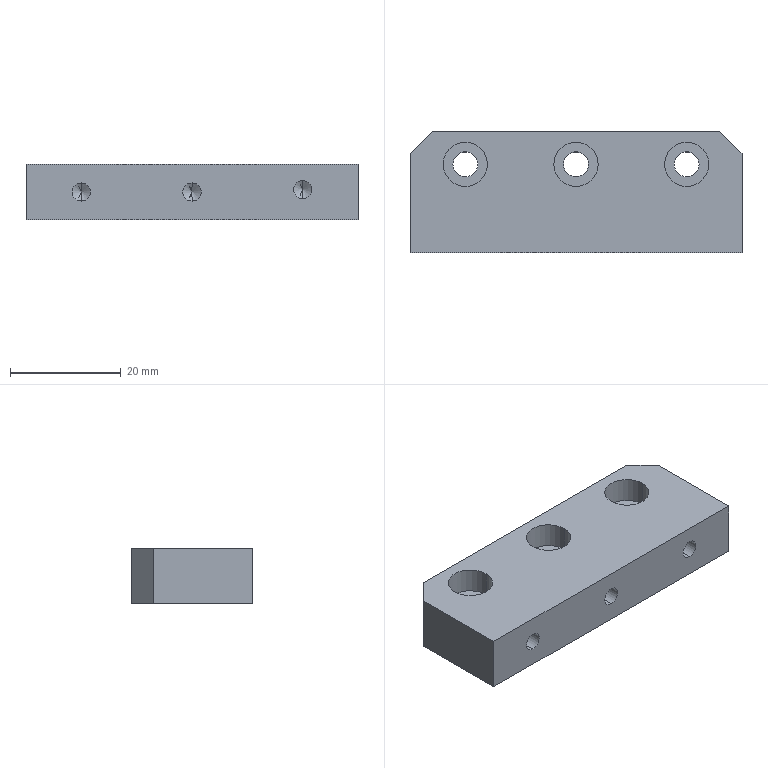Part | STEP file | MT-COMBO-119-S039 | 1 solid | 35 faces | box 60 x 22 x 10 mm | volume 11821 mm3 | cylinder 18 | plane 11 | cone 6 | commonest cylinder face diameters 3.3 x6 4.5 x6 8 x6
STEP:
#1=CARTESIAN_POINT('',(-24.,5.,5.4));
#2=VERTEX_POINT('',#1);
#3=CARTESIAN_POINT('',(-16.,5.,5.4));
#4=VERTEX_POINT('',#3);
#5=CARTESIAN_POINT('',(-20.,5.,5.4));
#6=DIRECTION('',(0.,0.,1.));
#7=DIRECTION('',(1.,0.,0.));
#8=AXIS2_PLACEMENT_3D('',#5,#6,#7);
#9=CIRCLE('',#8,4.);
#10=EDGE_CURVE('',#2,#4,#9,.T.);
#11=ORIENTED_EDGE('',*,*,#10,.F.);
#12=CARTESIAN_POINT('',(-24.,5.,10.));
#13=VERTEX_POINT('',#12);
#14=CARTESIAN_POINT('',(-24.,5.,10.));
#15=DIRECTION('',(0.,0.,1.));
#16=VECTOR('',#15,1000.);
#17=LINE('',#14,#16);
#18=EDGE_CURVE('',#2,#13,#17,.T.);
#19=ORIENTED_EDGE('',*,*,#18,.T.);
#20=CARTESIAN_POINT('',(-16.,5.,10.));
#21=VERTEX_POINT('',#20);
#22=CARTESIAN_POINT('',(-20.,5.,10.));
#23=DIRECTION('',(0.,0.,1.));
#24=DIRECTION('',(1.,0.,0.));
#25=AXIS2_PLACEMENT_3D('',#22,#23,#24);
#26=CIRCLE('',#25,4.);
#27=EDGE_CURVE('',#13,#21,#26,.T.);
#28=ORIENTED_EDGE('',*,*,#27,.T.);
#29=CARTESIAN_POINT('',(-16.,5.,10.));
#30=DIRECTION('',(0.,0.,1.));
#31=VECTOR('',#30,1000.);
#32=LINE('',#29,#31);
#33=EDGE_CURVE('',#4,#21,#32,.T.);
#34=ORIENTED_EDGE('',*,*,#33,.F.);
#35=EDGE_LOOP('',(#11,#19,#28,#34));
#36=FACE_OUTER_BOUND('',#35,.T.);
#37=CARTESIAN_POINT('',(-20.,5.,10.));
#38=DIRECTION('',(0.,0.,1.));
#39=DIRECTION('',(1.,0.,0.));
#40=AXIS2_PLACEMENT_3D('',#37,#38,#39);
#41=CYLINDRICAL_SURFACE('',#40,4.);
#42=ADVANCED_FACE('',(#36),#41,.F.);
#43=CARTESIAN_POINT('',(-22.25,5.,0.));
#44=VERTEX_POINT('',#43);
#45=CARTESIAN_POINT('',(-17.75,5.,0.));
#46=VERTEX_POINT('',#45);
#47=CARTESIAN_POINT('',(-20.,5.,0.));
#48=DIRECTION('',(0.,0.,1.));
#49=DIRECTION('',(1.,0.,0.));
#50=AXIS2_PLACEMENT_3D('',#47,#48,#49);
#51=CIRCLE('',#50,2.25);
#52=EDGE_CURVE('',#44,#46,#51,.T.);
#53=ORIENTED_EDGE('',*,*,#52,.F.);
#54=CARTESIAN_POINT('',(-22.25,5.,5.4));
#55=VERTEX_POINT('',#54);
#56=CARTESIAN_POINT('',(-22.25,5.,10.));
#57=DIRECTION('',(0.,0.,1.));
#58=VECTOR('',#57,1000.);
#59=LINE('',#56,#58);
#60=EDGE_CURVE('',#44,#55,#59,.T.);
#61=ORIENTED_EDGE('',*,*,#60,.T.);
#62=CARTESIAN_POINT('',(-17.75,5.,5.4));
#63=VERTEX_POINT('',#62);
#64=CARTESIAN_POINT('',(-20.,5.,5.4));
#65=DIRECTION('',(0.,0.,1.));
#66=DIRECTION('',(1.,0.,0.));
#67=AXIS2_PLACEMENT_3D('',#64,#65,#66);
#68=CIRCLE('',#67,2.25);
#69=EDGE_CURVE('',#55,#63,#68,.T.);
#70=ORIENTED_EDGE('',*,*,#69,.T.);
#71=CARTESIAN_POINT('',(-17.75,5.,10.));
#72=DIRECTION('',(0.,0.,1.));
#73=VECTOR('',#72,1000.);
#74=LINE('',#71,#73);
#75=EDGE_CURVE('',#46,#63,#74,.T.);
#76=ORIENTED_EDGE('',*,*,#75,.F.);
#77=EDGE_LOOP('',(#53,#61,#70,#76));
#78=FACE_OUTER_BOUND('',#77,.T.);
#79=CARTESIAN_POINT('',(-20.,5.,10.));
#80=DIRECTION('',(0.,0.,1.));
#81=DIRECTION('',(1.,0.,0.));
#82=AXIS2_PLACEMENT_3D('',#79,#80,#81);
#83=CYLINDRICAL_SURFACE('',#82,2.25);
#84=ADVANCED_FACE('',(#78),#83,.F.);
#85=CARTESIAN_POINT('',(-4.,5.,5.4));
#86=VERTEX_POINT('',#85);
#87=CARTESIAN_POINT('',(4.,5.,5.4));
#88=VERTEX_POINT('',#87);
#89=CARTESIAN_POINT('',(0.,5.,5.4));
#90=DIRECTION('',(0.,0.,1.));
#91=DIRECTION('',(1.,0.,0.));
#92=AXIS2_PLACEMENT_3D('',#89,#90,#91);
#93=CIRCLE('',#92,4.);
#94=EDGE_CURVE('',#86,#88,#93,.T.);
#95=ORIENTED_EDGE('',*,*,#94,.F.);
#96=CARTESIAN_POINT('',(-4.,5.,10.));
#97=VERTEX_POINT('',#96);
#98=CARTESIAN_POINT('',(-4.,5.,10.));
#99=DIRECTION('',(0.,0.,1.));
#100=VECTOR('',#99,1000.);
#101=LINE('',#98,#100);
#102=EDGE_CURVE('',#86,#97,#101,.T.);
#103=ORIENTED_EDGE('',*,*,#102,.T.);
#104=CARTESIAN_POINT('',(4.,5.,10.));
#105=VERTEX_POINT('',#104);
#106=CARTESIAN_POINT('',(0.,5.,10.));
#107=DIRECTION('',(0.,0.,1.));
#108=DIRECTION('',(1.,0.,0.));
#109=AXIS2_PLACEMENT_3D('',#106,#107,#108);
#110=CIRCLE('',#109,4.);
#111=EDGE_CURVE('',#97,#105,#110,.T.);
#112=ORIENTED_EDGE('',*,*,#111,.T.);
#113=CARTESIAN_POINT('',(4.,5.,10.));
#114=DIRECTION('',(0.,0.,1.));
#115=VECTOR('',#114,1000.);
#116=LINE('',#113,#115);
#117=EDGE_CURVE('',#88,#105,#116,.T.);
#118=ORIENTED_EDGE('',*,*,#117,.F.);
#119=EDGE_LOOP('',(#95,#103,#112,#118));
#120=FACE_OUTER_BOUND('',#119,.T.);
#121=CARTESIAN_POINT('',(0.,5.,10.));
#122=DIRECTION('',(0.,0.,1.));
#123=DIRECTION('',(1.,0.,0.));
#124=AXIS2_PLACEMENT_3D('',#121,#122,#123);
#125=CYLINDRICAL_SURFACE('',#124,4.);
#126=ADVANCED_FACE('',(#120),#125,.F.);
#127=CARTESIAN_POINT('',(-2.25,5.,0.));
#128=VERTEX_POINT('',#127);
#129=CARTESIAN_POINT('',(2.25,5.,0.));
#130=VERTEX_POINT('',#129);
#131=CARTESIAN_POINT('',(0.,5.,0.));
#132=DIRECTION('',(0.,0.,1.));
#133=DIRECTION('',(1.,0.,0.));
#134=AXIS2_PLACEMENT_3D('',#131,#132,#133);
#135=CIRCLE('',#134,2.25);
#136=EDGE_CURVE('',#128,#130,#135,.T.);
#137=ORIENTED_EDGE('',*,*,#136,.F.);
#138=CARTESIAN_POINT('',(-2.25,5.,5.4));
#139=VERTEX_POINT('',#138);
#140=CARTESIAN_POINT('',(-2.25,5.,10.));
#141=DIRECTION('',(0.,0.,1.));
#142=VECTOR('',#141,1000.);
#143=LINE('',#140,#142);
#144=EDGE_CURVE('',#128,#139,#143,.T.);
#145=ORIENTED_EDGE('',*,*,#144,.T.);
#146=CARTESIAN_POINT('',(2.25,5.,5.4));
#147=VERTEX_POINT('',#146);
#148=CARTESIAN_POINT('',(0.,5.,5.4));
#149=DIRECTION('',(0.,0.,1.));
#150=DIRECTION('',(1.,0.,0.));
#151=AXIS2_PLACEMENT_3D('',#148,#149,#150);
#152=CIRCLE('',#151,2.25);
#153=EDGE_CURVE('',#139,#147,#152,.T.);
#154=ORIENTED_EDGE('',*,*,#153,.T.);
#155=CARTESIAN_POINT('',(2.25,5.,10.));
#156=DIRECTION('',(0.,0.,1.));
#157=VECTOR('',#156,1000.);
#158=LINE('',#155,#157);
#159=EDGE_CURVE('',#130,#147,#158,.T.);
#160=ORIENTED_EDGE('',*,*,#159,.F.);
#161=EDGE_LOOP('',(#137,#145,#154,#160));
#162=FACE_OUTER_BOUND('',#161,.T.);
#163=CARTESIAN_POINT('',(0.,5.,10.));
#164=DIRECTION('',(0.,0.,1.));
#165=DIRECTION('',(1.,0.,0.));
#166=AXIS2_PLACEMENT_3D('',#163,#164,#165);
#167=CYLINDRICAL_SURFACE('',#166,2.25);
#168=ADVANCED_FACE('',(#162),#167,.F.);
#169=CARTESIAN_POINT('',(16.,5.,5.4));
#170=VERTEX_POINT('',#169);
#171=CARTESIAN_POINT('',(24.,5.,5.4));
#172=VERTEX_POINT('',#171);
#173=CARTESIAN_POINT('',(20.,5.,5.4));
#174=DIRECTION('',(0.,0.,1.));
#175=DIRECTION('',(1.,0.,0.));
#176=AXIS2_PLACEMENT_3D('',#173,#174,#175);
#177=CIRCLE('',#176,4.);
#178=EDGE_CURVE('',#170,#172,#177,.T.);
#179=ORIENTED_EDGE('',*,*,#178,.F.);
#180=CARTESIAN_POINT('',(16.,5.,10.));
#181=VERTEX_POINT('',#180);
#182=CARTESIAN_POINT('',(16.,5.,10.));
#183=DIRECTION('',(0.,0.,1.));
#184=VECTOR('',#183,1000.);
#185=LINE('',#182,#184);
#186=EDGE_CURVE('',#170,#181,#185,.T.);
#187=ORIENTED_EDGE('',*,*,#186,.T.);
#188=CARTESIAN_POINT('',(24.,5.,10.));
#189=VERTEX_POINT('',#188);
#190=CARTESIAN_POINT('',(20.,5.,10.));
#191=DIRECTION('',(0.,0.,1.));
#192=DIRECTION('',(1.,0.,0.));
#193=AXIS2_PLACEMENT_3D('',#190,#191,#192);
#194=CIRCLE('',#193,4.);
#195=EDGE_CURVE('',#181,#189,#194,.T.);
#196=ORIENTED_EDGE('',*,*,#195,.T.);
#197=CARTESIAN_POINT('',(24.,5.,10.));
#198=DIRECTION('',(0.,0.,1.));
#199=VECTOR('',#198,1000.);
#200=LINE('',#197,#199);
#201=EDGE_CURVE('',#172,#189,#200,.T.);
#202=ORIENTED_EDGE('',*,*,#201,.F.);
#203=EDGE_LOOP('',(#179,#187,#196,#202));
#204=FACE_OUTER_BOUND('',#203,.T.);
#205=CARTESIAN_POINT('',(20.,5.,10.));
#206=DIRECTION('',(0.,0.,1.));
#207=DIRECTION('',(1.,0.,0.));
#208=AXIS2_PLACEMENT_3D('',#205,#206,#207);
#209=CYLINDRICAL_SURFACE('',#208,4.);
#210=ADVANCED_FACE('',(#204),#209,.F.);
#211=CARTESIAN_POINT('',(17.75,5.,0.));
#212=VERTEX_POINT('',#211);
#213=CARTESIAN_POINT('',(22.25,5.,0.));
#214=VERTEX_POINT('',#213);
#215=CARTESIAN_POINT('',(20.,5.,0.));
#216=DIRECTION('',(0.,0.,1.));
#217=DIRECTION('',(1.,0.,0.));
#218=AXIS2_PLACEMENT_3D('',#215,#216,#217);
#219=CIRCLE('',#218,2.25);
#220=EDGE_CURVE('',#212,#214,#219,.T.);
#221=ORIENTED_EDGE('',*,*,#220,.F.);
#222=CARTESIAN_POINT('',(17.75,5.,5.4));
#223=VERTEX_POINT('',#222);
#224=CARTESIAN_POINT('',(17.75,5.,10.));
#225=DIRECTION('',(0.,0.,1.));
#226=VECTOR('',#225,1000.);
#227=LINE('',#224,#226);
#228=EDGE_CURVE('',#212,#223,#227,.T.);
#229=ORIENTED_EDGE('',*,*,#228,.T.);
#230=CARTESIAN_POINT('',(22.25,5.,5.4));
#231=VERTEX_POINT('',#230);
#232=CARTESIAN_POINT('',(20.,5.,5.4));
#233=DIRECTION('',(0.,0.,1.));
#234=DIRECTION('',(1.,0.,0.));
#235=AXIS2_PLACEMENT_3D('',#232,#233,#234);
#236=CIRCLE('',#235,2.25);
#237=EDGE_CURVE('',#223,#231,#236,.T.);
#238=ORIENTED_EDGE('',*,*,#237,.T.);
#239=CARTESIAN_POINT('',(22.25,5.,10.));
#240=DIRECTION('',(0.,0.,1.));
#241=VECTOR('',#240,1000.);
#242=LINE('',#239,#241);
#243=EDGE_CURVE('',#214,#231,#242,.T.);
#244=ORIENTED_EDGE('',*,*,#243,.F.);
#245=EDGE_LOOP('',(#221,#229,#238,#244));
#246=FACE_OUTER_BOUND('',#245,.T.);
#247=CARTESIAN_POINT('',(20.,5.,10.));
#248=DIRECTION('',(0.,0.,1.));
#249=DIRECTION('',(1.,0.,0.));
#250=AXIS2_PLACEMENT_3D('',#247,#248,#249);
#251=CYLINDRICAL_SURFACE('',#250,2.25);
#252=ADVANCED_FACE('',(#246),#251,.F.);
#253=CARTESIAN_POINT('',(-20.,-0.9,6.65));
#254=VERTEX_POINT('',#253);
#255=CARTESIAN_POINT('',(-20.,-0.9,3.35));
#256=VERTEX_POINT('',#255);
#257=CARTESIAN_POINT('',(-20.,-0.9,5.));
#258=DIRECTION('',(0.,-1.,0.));
#259=DIRECTION('',(0.,0.,-1.));
#260=AXIS2_PLACEMENT_3D('',#257,#258,#259);
#261=CIRCLE('',#260,1.65);
#262=EDGE_CURVE('',#254,#256,#261,.T.);
#263=ORIENTED_EDGE('',*,*,#262,.F.);
#264=CARTESIAN_POINT('',(-20.,-11.,6.65));
#265=VERTEX_POINT('',#264);
#266=CARTESIAN_POINT('',(-20.,-11.,6.65));
#267=DIRECTION('',(0.,-1.,0.));
#268=VECTOR('',#267,1000.);
#269=LINE('',#266,#268);
#270=EDGE_CURVE('',#254,#265,#269,.T.);
#271=ORIENTED_EDGE('',*,*,#270,.T.);
#272=CARTESIAN_POINT('',(-20.,-11.,3.35));
#273=VERTEX_POINT('',#272);
#274=CARTESIAN_POINT('',(-20.,-11.,5.));
#275=DIRECTION('',(0.,-1.,0.));
#276=DIRECTION('',(0.,0.,-1.));
#277=AXIS2_PLACEMENT_3D('',#274,#275,#276);
#278=CIRCLE('',#277,1.65);
#279=EDGE_CURVE('',#265,#273,#278,.T.);
#280=ORIENTED_EDGE('',*,*,#279,.T.);
#281=CARTESIAN_POINT('',(-20.,-11.,3.35));
#282=DIRECTION('',(0.,-1.,0.));
#283=VECTOR('',#282,1000.);
#284=LINE('',#281,#283);
#285=EDGE_CURVE('',#256,#273,#284,.T.);
#286=ORIENTED_EDGE('',*,*,#285,.F.);
#287=EDGE_LOOP('',(#263,#271,#280,#286));
#288=FACE_OUTER_BOUND('',#287,.T.);
#289=CARTESIAN_POINT('',(-20.,-11.,5.));
#290=DIRECTION('',(0.,-1.,0.));
#291=DIRECTION('',(0.,0.,-1.));
#292=AXIS2_PLACEMENT_3D('',#289,#290,#291);
#293=CYLINDRICAL_SURFACE('',#292,1.65);
#294=ADVANCED_FACE('',(#288),#293,.F.);
#295=CARTESIAN_POINT('',(-20.,0.09142,5.));
#296=VERTEX_POINT('',#295);
#297=CARTESIAN_POINT('',(-20.,-0.9,3.35));
#298=DIRECTION('',(0.,-0.515,-0.8572));
#299=VECTOR('',#298,1000.);
#300=LINE('',#297,#299);
#301=EDGE_CURVE('',#296,#256,#300,.T.);
#302=ORIENTED_EDGE('',*,*,#301,.F.);
#303=CARTESIAN_POINT('',(-20.,-0.9,6.65));
#304=DIRECTION('',(0.,-0.515,0.8572));
#305=VECTOR('',#304,1000.);
#306=LINE('',#303,#305);
#307=EDGE_CURVE('',#296,#254,#306,.T.);
#308=ORIENTED_EDGE('',*,*,#307,.T.);
#309=ORIENTED_EDGE('',*,*,#262,.T.);
#310=EDGE_LOOP('',(#302,#308,#309));
#311=FACE_OUTER_BOUND('',#310,.T.);
#312=CARTESIAN_POINT('',(-20.,-0.9,5.));
#313=DIRECTION('',(0.,-1.,0.));
#314=DIRECTION('',(0.,0.,-1.));
#315=AXIS2_PLACEMENT_3D('',#312,#313,#314);
#316=CONICAL_SURFACE('',#315,1.65,1.03);
#317=ADVANCED_FACE('',(#311),#316,.F.);
#318=CARTESIAN_POINT('',(0.,-0.9,6.65));
#319=VERTEX_POINT('',#318);
#320=CARTESIAN_POINT('',(0.,-0.9,3.35));
#321=VERTEX_POINT('',#320);
#322=CARTESIAN_POINT('',(0.,-0.9,5.));
#323=DIRECTION('',(0.,-1.,0.));
#324=DIRECTION('',(0.,0.,-1.));
#325=AXIS2_PLACEMENT_3D('',#322,#323,#324);
#326=CIRCLE('',#325,1.65);
#327=EDGE_CURVE('',#319,#321,#326,.T.);
#328=ORIENTED_EDGE('',*,*,#327,.F.);
#329=CARTESIAN_POINT('',(0.,-11.,6.65));
#330=VERTEX_POINT('',#329);
#331=CARTESIAN_POINT('',(0.,-11.,6.65));
#332=DIRECTION('',(0.,-1.,0.));
#333=VECTOR('',#332,1000.);
#334=LINE('',#331,#333);
#335=EDGE_CURVE('',#319,#330,#334,.T.);
#336=ORIENTED_EDGE('',*,*,#335,.T.);
#337=CARTESIAN_POINT('',(0.,-11.,3.35));
#338=VERTEX_POINT('',#337);
#339=CARTESIAN_POINT('',(0.,-11.,5.));
#340=DIRECTION('',(0.,-1.,0.));
#341=DIRECTION('',(0.,0.,-1.));
#342=AXIS2_PLACEMENT_3D('',#339,#340,#341);
#343=CIRCLE('',#342,1.65);
#344=EDGE_CURVE('',#330,#338,#343,.T.);
#345=ORIENTED_EDGE('',*,*,#344,.T.);
#346=CARTESIAN_POINT('',(0.,-11.,3.35));
#347=DIRECTION('',(0.,-1.,0.));
#348=VECTOR('',#347,1000.);
#349=LINE('',#346,#348);
#350=EDGE_CURVE('',#321,#338,#349,.T.);
#351=ORIENTED_EDGE('',*,*,#350,.F.);
#352=EDGE_LOOP('',(#328,#336,#345,#351));
#353=FACE_OUTER_BOUND('',#352,.T.);
#354=CARTESIAN_POINT('',(0.,-11.,5.));
#355=DIRECTION('',(0.,-1.,0.));
#356=DIRECTION('',(0.,0.,-1.));
#357=AXIS2_PLACEMENT_3D('',#354,#355,#356);
#358=CYLINDRICAL_SURFACE('',#357,1.65);
#359=ADVANCED_FACE('',(#353),#358,.F.);
#360=CARTESIAN_POINT('',(0.,0.09142,5.));
#361=VERTEX_POINT('',#360);
#362=CARTESIAN_POINT('',(0.,-0.9,3.35));
#363=DIRECTION('',(0.,-0.515,-0.8572));
#364=VECTOR('',#363,1000.);
#365=LINE('',#362,#364);
#366=EDGE_CURVE('',#361,#321,#365,.T.);
#367=ORIENTED_EDGE('',*,*,#366,.F.);
#368=CARTESIAN_POINT('',(0.,-0.9,6.65));
#369=DIRECTION('',(0.,-0.515,0.8572));
#370=VECTOR('',#369,1000.);
#371=LINE('',#368,#370);
#372=EDGE_CURVE('',#361,#319,#371,.T.);
#373=ORIENTED_EDGE('',*,*,#372,.T.);
#374=ORIENTED_EDGE('',*,*,#327,.T.);
#375=EDGE_LOOP('',(#367,#373,#374));
#376=FACE_OUTER_BOUND('',#375,.T.);
#377=CARTESIAN_POINT('',(0.,-0.9,5.));
#378=DIRECTION('',(0.,-1.,0.));
#379=DIRECTION('',(0.,0.,-1.));
#380=AXIS2_PLACEMENT_3D('',#377,#378,#379);
#381=CONICAL_SURFACE('',#380,1.65,1.03);
#382=ADVANCED_FACE('',(#376),#381,.F.);
#383=CARTESIAN_POINT('',(20.,-0.9,7.072));
#384=VERTEX_POINT('',#383);
#385=CARTESIAN_POINT('',(20.,-0.9,3.772));
#386=VERTEX_POINT('',#385);
#387=CARTESIAN_POINT('',(20.,-0.9,5.422));
#388=DIRECTION('',(0.,-1.,0.));
#389=DIRECTION('',(0.,0.,-1.));
#390=AXIS2_PLACEMENT_3D('',#387,#388,#389);
#391=CIRCLE('',#390,1.65);
#392=EDGE_CURVE('',#384,#386,#391,.T.);
#393=ORIENTED_EDGE('',*,*,#392,.F.);
#394=CARTESIAN_POINT('',(20.,-11.,7.072));
#395=VERTEX_POINT('',#394);
#396=CARTESIAN_POINT('',(20.,-11.,7.072));
#397=DIRECTION('',(0.,-1.,0.));
#398=VECTOR('',#397,1000.);
#399=LINE('',#396,#398);
#400=EDGE_CURVE('',#384,#395,#399,.T.);
#401=ORIENTED_EDGE('',*,*,#400,.T.);
#402=CARTESIAN_POINT('',(20.,-11.,3.772));
#403=VERTEX_POINT('',#402);
#404=CARTESIAN_POINT('',(20.,-11.,5.422));
#405=DIRECTION('',(0.,-1.,0.));
#406=DIRECTION('',(0.,0.,-1.));
#407=AXIS2_PLACEMENT_3D('',#404,#405,#406);
#408=CIRCLE('',#407,1.65);
#409=EDGE_CURVE('',#395,#403,#408,.T.);
#410=ORIENTED_EDGE('',*,*,#409,.T.);
#411=CARTESIAN_POINT('',(20.,-11.,3.772));
#412=DIRECTION('',(0.,-1.,0.));
#413=VECTOR('',#412,1000.);
#414=LINE('',#411,#413);
#415=EDGE_CURVE('',#386,#403,#414,.T.);
#416=ORIENTED_EDGE('',*,*,#415,.F.);
#417=EDGE_LOOP('',(#393,#401,#410,#416));
#418=FACE_OUTER_BOUND('',#417,.T.);
#419=CARTESIAN_POINT('',(20.,-11.,5.422));
#420=DIRECTION('',(0.,-1.,0.));
#421=DIRECTION('',(0.,0.,-1.));
#422=AXIS2_PLACEMENT_3D('',#419,#420,#421);
#423=CYLINDRICAL_SURFACE('',#422,1.65);
#424=ADVANCED_FACE('',(#418),#423,.F.);
#425=CARTESIAN_POINT('',(20.,0.09142,5.422));
#426=VERTEX_POINT('',#425);
#427=CARTESIAN_POINT('',(20.,-0.9,3.772));
#428=DIRECTION('',(0.,-0.515,-0.8572));
#429=VECTOR('',#428,1000.);
#430=LINE('',#427,#429);
#431=EDGE_CURVE('',#426,#386,#430,.T.);
#432=ORIENTED_EDGE('',*,*,#431,.F.);
#433=CARTESIAN_POINT('',(20.,-0.9,7.072));
#434=DIRECTION('',(0.,-0.515,0.8572));
#435=VECTOR('',#434,1000.);
#436=LINE('',#433,#435);
#437=EDGE_CURVE('',#426,#384,#436,.T.);
#438=ORIENTED_EDGE('',*,*,#437,.T.);
#439=ORIENTED_EDGE('',*,*,#392,.T.);
#440=EDGE_LOOP('',(#432,#438,#439));
#441=FACE_OUTER_BOUND('',#440,.T.);
#442=CARTESIAN_POINT('',(20.,-0.9,5.422));
#443=DIRECTION('',(0.,-1.,0.));
#444=DIRECTION('',(0.,0.,-1.));
#445=AXIS2_PLACEMENT_3D('',#442,#443,#444);
#446=CONICAL_SURFACE('',#445,1.65,1.03);
#447=ADVANCED_FACE('',(#441),#446,.F.);
#448=CARTESIAN_POINT('',(-30.,7.,10.));
#449=VERTEX_POINT('',#448);
#450=CARTESIAN_POINT('',(-30.,-11.,10.));
#451=VERTEX_POINT('',#450);
#452=CARTESIAN_POINT('',(-30.,-11.,10.));
#453=DIRECTION('',(0.,-1.,0.));
#454=VECTOR('',#453,1000.);
#455=LINE('',#452,#454);
#456=EDGE_CURVE('',#449,#451,#455,.T.);
#457=ORIENTED_EDGE('',*,*,#456,.F.);
#458=CARTESIAN_POINT('',(-30.,7.,0.));
#459=VERTEX_POINT('',#458);
#460=CARTESIAN_POINT('',(-30.,7.,10.));
#461=DIRECTION('',(0.,0.,-1.));
#462=VECTOR('',#461,1000.);
#463=LINE('',#460,#462);
#464=EDGE_CURVE('',#449,#459,#463,.T.);
#465=ORIENTED_EDGE('',*,*,#464,.T.);
#466=CARTESIAN_POINT('',(-30.,-11.,0.));
#467=VERTEX_POINT('',#466);
#468=CARTESIAN_POINT('',(-30.,-11.,0.));
#469=DIRECTION('',(0.,-1.,0.));
#470=VECTOR('',#469,1000.);
#471=LINE('',#468,#470);
#472=EDGE_CURVE('',#459,#467,#471,.T.);
#473=ORIENTED_EDGE('',*,*,#472,.T.);
#474=CARTESIAN_POINT('',(-30.,-11.,10.));
#475=DIRECTION('',(0.,0.,-1.));
#476=VECTOR('',#475,1000.);
#477=LINE('',#474,#476);
#478=EDGE_CURVE('',#451,#467,#477,.T.);
#479=ORIENTED_EDGE('',*,*,#478,.F.);
#480=EDGE_LOOP('',(#457,#465,#473,#479));
#481=FACE_OUTER_BOUND('',#480,.T.);
#482=CARTESIAN_POINT('',(-30.,-11.,10.));
#483=DIRECTION('',(1.,0.,0.));
#484=DIRECTION('',(0.,0.,-1.));
#485=AXIS2_PLACEMENT_3D('',#482,#483,#484);
#486=PLANE('',#485);
#487=ADVANCED_FACE('',(#481),#486,.F.);
#488=CARTESIAN_POINT('',(-20.,-11.,5.));
#489=DIRECTION('',(0.,-1.,0.));
#490=DIRECTION('',(0.,0.,-1.));
#491=AXIS2_PLACEMENT_3D('',#488,#489,#490);
#492=CIRCLE('',#491,1.65);
#493=EDGE_CURVE('',#273,#265,#492,.T.);
#494=ORIENTED_EDGE('',*,*,#493,.F.);
#495=ORIENTED_EDGE('',*,*,#279,.F.);
#496=EDGE_LOOP('',(#494,#495));
#497=FACE_BOUND('',#496,.T.);
#498=CARTESIAN_POINT('',(0.,-11.,5.));
#499=DIRECTION('',(0.,-1.,0.));
#500=DIRECTION('',(0.,0.,-1.));
#501=AXIS2_PLACEMENT_3D('',#498,#499,#500);
#502=CIRCLE('',#501,1.65);
#503=EDGE_CURVE('',#338,#330,#502,.T.);
#504=ORIENTED_EDGE('',*,*,#503,.F.);
#505=ORIENTED_EDGE('',*,*,#344,.F.);
#506=EDGE_LOOP('',(#504,#505));
#507=FACE_BOUND('',#506,.T.);
#508=CARTESIAN_POINT('',(20.,-11.,5.422));
#509=DIRECTION('',(0.,-1.,0.));
#510=DIRECTION('',(0.,0.,-1.));
#511=AXIS2_PLACEMENT_3D('',#508,#509,#510);
#512=CIRCLE('',#511,1.65);
#513=EDGE_CURVE('',#403,#395,#512,.T.);
#514=ORIENTED_EDGE('',*,*,#513,.F.);
#515=ORIENTED_EDGE('',*,*,#409,.F.);
#516=EDGE_LOOP('',(#514,#515));
#517=FACE_BOUND('',#516,.T.);
#518=CARTESIAN_POINT('',(30.,-11.,0.));
#519=VERTEX_POINT('',#518);
#520=CARTESIAN_POINT('',(30.,-11.,0.));
#521=DIRECTION('',(1.,0.,0.));
#522=VECTOR('',#521,1000.);
#523=LINE('',#520,#522);
#524=EDGE_CURVE('',#467,#519,#523,.T.);
#525=ORIENTED_EDGE('',*,*,#524,.T.);
#526=CARTESIAN_POINT('',(30.,-11.,10.));
#527=VERTEX_POINT('',#526);
#528=CARTESIAN_POINT('',(30.,-11.,10.));
#529=DIRECTION('',(0.,0.,-1.));
#530=VECTOR('',#529,1000.);
#531=LINE('',#528,#530);
#532=EDGE_CURVE('',#527,#519,#531,.T.);
#533=ORIENTED_EDGE('',*,*,#532,.F.);
#534=CARTESIAN_POINT('',(30.,-11.,10.));
#535=DIRECTION('',(1.,0.,0.));
#536=VECTOR('',#535,1000.);
#537=LINE('',#534,#536);
#538=EDGE_CURVE('',#451,#527,#537,.T.);
#539=ORIENTED_EDGE('',*,*,#538,.F.);
#540=ORIENTED_EDGE('',*,*,#478,.T.);
#541=EDGE_LOOP('',(#525,#533,#539,#540));
#542=FACE_OUTER_BOUND('',#541,.T.);
#543=CARTESIAN_POINT('',(30.,-11.,10.));
#544=DIRECTION('',(0.,1.,0.));
#545=DIRECTION('',(0.,0.,1.));
#546=AXIS2_PLACEMENT_3D('',#543,#544,#545);
#547=PLANE('',#546);
#548=ADVANCED_FACE('',(#497,#507,#517,#542),#547,.F.);
#549=CARTESIAN_POINT('',(30.,7.,0.));
#550=VERTEX_POINT('',#549);
#551=CARTESIAN_POINT('',(30.,-11.,0.));
#552=DIRECTION('',(0.,1.,0.));
#553=VECTOR('',#552,1000.);
#554=LINE('',#551,#553);
#555=EDGE_CURVE('',#519,#550,#554,.T.);
#556=ORIENTED_EDGE('',*,*,#555,.T.);
#557=CARTESIAN_POINT('',(30.,7.,10.));
#558=VERTEX_POINT('',#557);
#559=CARTESIAN_POINT('',(30.,7.,10.));
#560=DIRECTION('',(0.,0.,1.));
#561=VECTOR('',#560,1000.);
#562=LINE('',#559,#561);
#563=EDGE_CURVE('',#550,#558,#562,.T.);
#564=ORIENTED_EDGE('',*,*,#563,.T.);
#565=CARTESIAN_POINT('',(30.,-11.,10.));
#566=DIRECTION('',(0.,1.,0.));
#567=VECTOR('',#566,1000.);
#568=LINE('',#565,#567);
#569=EDGE_CURVE('',#527,#558,#568,.T.);
#570=ORIENTED_EDGE('',*,*,#569,.F.);
#571=ORIENTED_EDGE('',*,*,#532,.T.);
#572=EDGE_LOOP('',(#556,#564,#570,#571));
#573=FACE_OUTER_BOUND('',#572,.T.);
#574=CARTESIAN_POINT('',(30.,-11.,10.));
#575=DIRECTION('',(-1.,0.,0.));
#576=DIRECTION('',(0.,0.,1.));
#577=AXIS2_PLACEMENT_3D('',#574,#575,#576);
#578=PLANE('',#577);
#579=ADVANCED_FACE('',(#573),#578,.F.);
#580=CARTESIAN_POINT('',(26.,11.,10.));
#581=VERTEX_POINT('',#580);
#582=CARTESIAN_POINT('',(-26.,11.,10.));
#583=VERTEX_POINT('',#582);
#584=CARTESIAN_POINT('',(30.,11.,10.));
#585=DIRECTION('',(-1.,0.,0.));
#586=VECTOR('',#585,1000.);
#587=LINE('',#584,#586);
#588=EDGE_CURVE('',#581,#583,#587,.T.);
#589=ORIENTED_EDGE('',*,*,#588,.F.);
#590=CARTESIAN_POINT('',(26.,11.,0.));
#591=VERTEX_POINT('',#590);
#592=CARTESIAN_POINT('',(26.,11.,10.));
#593=DIRECTION('',(0.,0.,-1.));
#594=VECTOR('',#593,1000.);
#595=LINE('',#592,#594);
#596=EDGE_CURVE('',#581,#591,#595,.T.);
#597=ORIENTED_EDGE('',*,*,#596,.T.);
#598=CARTESIAN_POINT('',(-26.,11.,0.));
#599=VERTEX_POINT('',#598);
#600=CARTESIAN_POINT('',(30.,11.,0.));
#601=DIRECTION('',(-1.,0.,0.));
#602=VECTOR('',#601,1000.);
#603=LINE('',#600,#602);
#604=EDGE_CURVE('',#591,#599,#603,.T.);
#605=ORIENTED_EDGE('',*,*,#604,.T.);
#606=CARTESIAN_POINT('',(-26.,11.,10.));
#607=DIRECTION('',(0.,0.,1.));
#608=VECTOR('',#607,1000.);
#609=LINE('',#606,#608);
#610=EDGE_CURVE('',#599,#583,#609,.T.);
#611=ORIENTED_EDGE('',*,*,#610,.T.);
#612=EDGE_LOOP('',(#589,#597,#605,#611));
#613=FACE_OUTER_BOUND('',#612,.T.);
#614=CARTESIAN_POINT('',(30.,11.,10.));
#615=DIRECTION('',(0.,-1.,0.));
#616=DIRECTION('',(0.,0.,-1.));
#617=AXIS2_PLACEMENT_3D('',#614,#615,#616);
#618=PLANE('',#617);
#619=ADVANCED_FACE('',(#613),#618,.F.);
#620=CARTESIAN_POINT('',(-20.,5.,10.));
#621=DIRECTION('',(0.,0.,1.));
#622=DIRECTION('',(1.,0.,0.));
#623=AXIS2_PLACEMENT_3D('',#620,#621,#622);
#624=CIRCLE('',#623,4.);
#625=EDGE_CURVE('',#21,#13,#624,.T.);
#626=ORIENTED_EDGE('',*,*,#625,.F.);
#627=ORIENTED_EDGE('',*,*,#27,.F.);
#628=EDGE_LOOP('',(#626,#627));
#629=FACE_BOUND('',#628,.T.);
#630=CARTESIAN_POINT('',(0.,5.,10.));
#631=DIRECTION('',(0.,0.,1.));
#632=DIRECTION('',(1.,0.,0.));
#633=AXIS2_PLACEMENT_3D('',#630,#631,#632);
#634=CIRCLE('',#633,4.);
#635=EDGE_CURVE('',#105,#97,#634,.T.);
#636=ORIENTED_EDGE('',*,*,#635,.F.);
#637=ORIENTED_EDGE('',*,*,#111,.F.);
#638=EDGE_LOOP('',(#636,#637));
#639=FACE_BOUND('',#638,.T.);
#640=CARTESIAN_POINT('',(20.,5.,10.));
#641=DIRECTION('',(0.,0.,1.));
#642=DIRECTION('',(1.,0.,0.));
#643=AXIS2_PLACEMENT_3D('',#640,#641,#642);
#644=CIRCLE('',#643,4.);
#645=EDGE_CURVE('',#189,#181,#644,.T.);
#646=ORIENTED_EDGE('',*,*,#645,.F.);
#647=ORIENTED_EDGE('',*,*,#195,.F.);
#648=EDGE_LOOP('',(#646,#647));
#649=FACE_BOUND('',#648,.T.);
#650=ORIENTED_EDGE('',*,*,#569,.T.);
#651=CARTESIAN_POINT('',(18.5,18.5,10.));
#652=DIRECTION('',(-0.7071,0.7071,0.));
#653=VECTOR('',#652,1000.);
#654=LINE('',#651,#653);
#655=EDGE_CURVE('',#558,#581,#654,.T.);
#656=ORIENTED_EDGE('',*,*,#655,.T.);
#657=ORIENTED_EDGE('',*,*,#588,.T.);
#658=CARTESIAN_POINT('',(-18.5,18.5,10.));
#659=DIRECTION('',(-0.7071,-0.7071,0.));
#660=VECTOR('',#659,1000.);
#661=LINE('',#658,#660);
#662=EDGE_CURVE('',#583,#449,#661,.T.);
#663=ORIENTED_EDGE('',*,*,#662,.T.);
#664=ORIENTED_EDGE('',*,*,#456,.T.);
#665=ORIENTED_EDGE('',*,*,#538,.T.);
#666=EDGE_LOOP('',(#650,#656,#657,#663,#664,#665));
#667=FACE_OUTER_BOUND('',#666,.T.);
#668=CARTESIAN_POINT('',(0.,0.,10.));
#669=DIRECTION('',(0.,0.,1.));
#670=DIRECTION('',(1.,0.,0.));
#671=AXIS2_PLACEMENT_3D('',#668,#669,#670);
#672=PLANE('',#671);
#673=ADVANCED_FACE('',(#629,#639,#649,#667),#672,.T.);
#674=CARTESIAN_POINT('',(-20.,5.,0.));
#675=DIRECTION('',(0.,0.,1.));
#676=DIRECTION('',(1.,0.,0.));
#677=AXIS2_PLACEMENT_3D('',#674,#675,#676);
#678=CIRCLE('',#677,2.25);
#679=EDGE_CURVE('',#46,#44,#678,.T.);
#680=ORIENTED_EDGE('',*,*,#679,.T.);
#681=ORIENTED_EDGE('',*,*,#52,.T.);
#682=EDGE_LOOP('',(#680,#681));
#683=FACE_BOUND('',#682,.T.);
#684=CARTESIAN_POINT('',(0.,5.,0.));
#685=DIRECTION('',(0.,0.,1.));
#686=DIRECTION('',(1.,0.,0.));
#687=AXIS2_PLACEMENT_3D('',#684,#685,#686);
#688=CIRCLE('',#687,2.25);
#689=EDGE_CURVE('',#130,#128,#688,.T.);
#690=ORIENTED_EDGE('',*,*,#689,.T.);
#691=ORIENTED_EDGE('',*,*,#136,.T.);
#692=EDGE_LOOP('',(#690,#691));
#693=FACE_BOUND('',#692,.T.);
#694=CARTESIAN_POINT('',(20.,5.,0.));
#695=DIRECTION('',(0.,0.,1.));
#696=DIRECTION('',(1.,0.,0.));
#697=AXIS2_PLACEMENT_3D('',#694,#695,#696);
#698=CIRCLE('',#697,2.25);
#699=EDGE_CURVE('',#214,#212,#698,.T.);
#700=ORIENTED_EDGE('',*,*,#699,.T.);
#701=ORIENTED_EDGE('',*,*,#220,.T.);
#702=EDGE_LOOP('',(#700,#701));
#703=FACE_BOUND('',#702,.T.);
#704=ORIENTED_EDGE('',*,*,#604,.F.);
#705=CARTESIAN_POINT('',(26.,11.,0.));
#706=DIRECTION('',(0.7071,-0.7071,0.));
#707=VECTOR('',#706,1000.);
#708=LINE('',#705,#707);
#709=EDGE_CURVE('',#591,#550,#708,.T.);
#710=ORIENTED_EDGE('',*,*,#709,.T.);
#711=ORIENTED_EDGE('',*,*,#555,.F.);
#712=ORIENTED_EDGE('',*,*,#524,.F.);
#713=ORIENTED_EDGE('',*,*,#472,.F.);
#714=CARTESIAN_POINT('',(-30.,7.,0.));
#715=DIRECTION('',(0.7071,0.7071,0.));
#716=VECTOR('',#715,1000.);
#717=LINE('',#714,#716);
#718=EDGE_CURVE('',#459,#599,#717,.T.);
#719=ORIENTED_EDGE('',*,*,#718,.T.);
#720=EDGE_LOOP('',(#704,#710,#711,#712,#713,#719));
#721=FACE_OUTER_BOUND('',#720,.T.);
#722=CARTESIAN_POINT('',(0.,0.,0.));
#723=DIRECTION('',(0.,0.,1.));
#724=DIRECTION('',(1.,0.,0.));
#725=AXIS2_PLACEMENT_3D('',#722,#723,#724);
#726=PLANE('',#725);
#727=ADVANCED_FACE('',(#683,#693,#703,#721),#726,.F.);
#728=ORIENTED_EDGE('',*,*,#437,.F.);
#729=ORIENTED_EDGE('',*,*,#431,.T.);
#730=CARTESIAN_POINT('',(20.,-0.9,5.422));
#731=DIRECTION('',(0.,-1.,0.));
#732=DIRECTION('',(0.,0.,-1.));
#733=AXIS2_PLACEMENT_3D('',#730,#731,#732);
#734=CIRCLE('',#733,1.65);
#735=EDGE_CURVE('',#386,#384,#734,.T.);
#736=ORIENTED_EDGE('',*,*,#735,.T.);
#737=EDGE_LOOP('',(#728,#729,#736));
#738=FACE_OUTER_BOUND('',#737,.T.);
#739=CARTESIAN_POINT('',(20.,-0.9,5.422));
#740=DIRECTION('',(0.,-1.,0.));
#741=DIRECTION('',(0.,0.,-1.));
#742=AXIS2_PLACEMENT_3D('',#739,#740,#741);
#743=CONICAL_SURFACE('',#742,1.65,1.03);
#744=ADVANCED_FACE('',(#738),#743,.F.);
#745=ORIENTED_EDGE('',*,*,#400,.F.);
#746=ORIENTED_EDGE('',*,*,#735,.F.);
#747=ORIENTED_EDGE('',*,*,#415,.T.);
#748=ORIENTED_EDGE('',*,*,#513,.T.);
#749=EDGE_LOOP('',(#745,#746,#747,#748));
#750=FACE_OUTER_BOUND('',#749,.T.);
#751=CARTESIAN_POINT('',(20.,-11.,5.422));
#752=DIRECTION('',(0.,-1.,0.));
#753=DIRECTION('',(0.,0.,-1.));
#754=AXIS2_PLACEMENT_3D('',#751,#752,#753);
#755=CYLINDRICAL_SURFACE('',#754,1.65);
#756=ADVANCED_FACE('',(#750),#755,.F.);
#757=ORIENTED_EDGE('',*,*,#372,.F.);
#758=ORIENTED_EDGE('',*,*,#366,.T.);
#759=CARTESIAN_POINT('',(0.,-0.9,5.));
#760=DIRECTION('',(0.,-1.,0.));
#761=DIRECTION('',(0.,0.,-1.));
#762=AXIS2_PLACEMENT_3D('',#759,#760,#761);
#763=CIRCLE('',#762,1.65);
#764=EDGE_CURVE('',#321,#319,#763,.T.);
#765=ORIENTED_EDGE('',*,*,#764,.T.);
#766=EDGE_LOOP('',(#757,#758,#765));
#767=FACE_OUTER_BOUND('',#766,.T.);
#768=CARTESIAN_POINT('',(0.,-0.9,5.));
#769=DIRECTION('',(0.,-1.,0.));
#770=DIRECTION('',(0.,0.,-1.));
#771=AXIS2_PLACEMENT_3D('',#768,#769,#770);
#772=CONICAL_SURFACE('',#771,1.65,1.03);
#773=ADVANCED_FACE('',(#767),#772,.F.);
#774=ORIENTED_EDGE('',*,*,#335,.F.);
#775=ORIENTED_EDGE('',*,*,#764,.F.);
#776=ORIENTED_EDGE('',*,*,#350,.T.);
#777=ORIENTED_EDGE('',*,*,#503,.T.);
#778=EDGE_LOOP('',(#774,#775,#776,#777));
#779=FACE_OUTER_BOUND('',#778,.T.);
#780=CARTESIAN_POINT('',(0.,-11.,5.));
#781=DIRECTION('',(0.,-1.,0.));
#782=DIRECTION('',(0.,0.,-1.));
#783=AXIS2_PLACEMENT_3D('',#780,#781,#782);
#784=CYLINDRICAL_SURFACE('',#783,1.65);
#785=ADVANCED_FACE('',(#779),#784,.F.);
#786=ORIENTED_EDGE('',*,*,#307,.F.);
#787=ORIENTED_EDGE('',*,*,#301,.T.);
#788=CARTESIAN_POINT('',(-20.,-0.9,5.));
#789=DIRECTION('',(0.,-1.,0.));
#790=DIRECTION('',(0.,0.,-1.));
#791=AXIS2_PLACEMENT_3D('',#788,#789,#790);
#792=CIRCLE('',#791,1.65);
#793=EDGE_CURVE('',#256,#254,#792,.T.);
#794=ORIENTED_EDGE('',*,*,#793,.T.);
#795=EDGE_LOOP('',(#786,#787,#794));
#796=FACE_OUTER_BOUND('',#795,.T.);
#797=CARTESIAN_POINT('',(-20.,-0.9,5.));
#798=DIRECTION('',(0.,-1.,0.));
#799=DIRECTION('',(0.,0.,-1.));
#800=AXIS2_PLACEMENT_3D('',#797,#798,#799);
#801=CONICAL_SURFACE('',#800,1.65,1.03);
#802=ADVANCED_FACE('',(#796),#801,.F.);
#803=ORIENTED_EDGE('',*,*,#270,.F.);
#804=ORIENTED_EDGE('',*,*,#793,.F.);
#805=ORIENTED_EDGE('',*,*,#285,.T.);
#806=ORIENTED_EDGE('',*,*,#493,.T.);
#807=EDGE_LOOP('',(#803,#804,#805,#806));
#808=FACE_OUTER_BOUND('',#807,.T.);
#809=CARTESIAN_POINT('',(-20.,-11.,5.));
#810=DIRECTION('',(0.,-1.,0.));
#811=DIRECTION('',(0.,0.,-1.));
#812=AXIS2_PLACEMENT_3D('',#809,#810,#811);
#813=CYLINDRICAL_SURFACE('',#812,1.65);
#814=ADVANCED_FACE('',(#808),#813,.F.);
#815=ORIENTED_EDGE('',*,*,#228,.F.);
#816=ORIENTED_EDGE('',*,*,#699,.F.);
#817=ORIENTED_EDGE('',*,*,#243,.T.);
#818=CARTESIAN_POINT('',(20.,5.,5.4));
#819=DIRECTION('',(0.,0.,1.));
#820=DIRECTION('',(1.,0.,0.));
#821=AXIS2_PLACEMENT_3D('',#818,#819,#820);
#822=CIRCLE('',#821,2.25);
#823=EDGE_CURVE('',#231,#223,#822,.T.);
#824=ORIENTED_EDGE('',*,*,#823,.T.);
#825=EDGE_LOOP('',(#815,#816,#817,#824));
#826=FACE_OUTER_BOUND('',#825,.T.);
#827=CARTESIAN_POINT('',(20.,5.,10.));
#828=DIRECTION('',(0.,0.,1.));
#829=DIRECTION('',(1.,0.,0.));
#830=AXIS2_PLACEMENT_3D('',#827,#828,#829);
#831=CYLINDRICAL_SURFACE('',#830,2.25);
#832=ADVANCED_FACE('',(#826),#831,.F.);
#833=ORIENTED_EDGE('',*,*,#823,.F.);
#834=ORIENTED_EDGE('',*,*,#237,.F.);
#835=EDGE_LOOP('',(#833,#834));
#836=FACE_BOUND('',#835,.T.);
#837=CARTESIAN_POINT('',(20.,5.,5.4));
#838=DIRECTION('',(0.,0.,1.));
#839=DIRECTION('',(1.,0.,0.));
#840=AXIS2_PLACEMENT_3D('',#837,#838,#839);
#841=CIRCLE('',#840,4.);
#842=EDGE_CURVE('',#172,#170,#841,.T.);
#843=ORIENTED_EDGE('',*,*,#842,.T.);
#844=ORIENTED_EDGE('',*,*,#178,.T.);
#845=EDGE_LOOP('',(#843,#844));
#846=FACE_OUTER_BOUND('',#845,.T.);
#847=CARTESIAN_POINT('',(22.25,5.,5.4));
#848=DIRECTION('',(0.,0.,-1.));
#849=DIRECTION('',(-1.,0.,0.));
#850=AXIS2_PLACEMENT_3D('',#847,#848,#849);
#851=PLANE('',#850);
#852=ADVANCED_FACE('',(#836,#846),#851,.F.);
#853=ORIENTED_EDGE('',*,*,#186,.F.);
#854=ORIENTED_EDGE('',*,*,#842,.F.);
#855=ORIENTED_EDGE('',*,*,#201,.T.);
#856=ORIENTED_EDGE('',*,*,#645,.T.);
#857=EDGE_LOOP('',(#853,#854,#855,#856));
#858=FACE_OUTER_BOUND('',#857,.T.);
#859=CARTESIAN_POINT('',(20.,5.,10.));
#860=DIRECTION('',(0.,0.,1.));
#861=DIRECTION('',(1.,0.,0.));
#862=AXIS2_PLACEMENT_3D('',#859,#860,#861);
#863=CYLINDRICAL_SURFACE('',#862,4.);
#864=ADVANCED_FACE('',(#858),#863,.F.);
#865=ORIENTED_EDGE('',*,*,#144,.F.);
#866=ORIENTED_EDGE('',*,*,#689,.F.);
#867=ORIENTED_EDGE('',*,*,#159,.T.);
#868=CARTESIAN_POINT('',(0.,5.,5.4));
#869=DIRECTION('',(0.,0.,1.));
#870=DIRECTION('',(1.,0.,0.));
#871=AXIS2_PLACEMENT_3D('',#868,#869,#870);
#872=CIRCLE('',#871,2.25);
#873=EDGE_CURVE('',#147,#139,#872,.T.);
#874=ORIENTED_EDGE('',*,*,#873,.T.);
#875=EDGE_LOOP('',(#865,#866,#867,#874));
#876=FACE_OUTER_BOUND('',#875,.T.);
#877=CARTESIAN_POINT('',(0.,5.,10.));
#878=DIRECTION('',(0.,0.,1.));
#879=DIRECTION('',(1.,0.,0.));
#880=AXIS2_PLACEMENT_3D('',#877,#878,#879);
#881=CYLINDRICAL_SURFACE('',#880,2.25);
#882=ADVANCED_FACE('',(#876),#881,.F.);
#883=ORIENTED_EDGE('',*,*,#873,.F.);
#884=ORIENTED_EDGE('',*,*,#153,.F.);
#885=EDGE_LOOP('',(#883,#884));
#886=FACE_BOUND('',#885,.T.);
#887=CARTESIAN_POINT('',(0.,5.,5.4));
#888=DIRECTION('',(0.,0.,1.));
#889=DIRECTION('',(1.,0.,0.));
#890=AXIS2_PLACEMENT_3D('',#887,#888,#889);
#891=CIRCLE('',#890,4.);
#892=EDGE_CURVE('',#88,#86,#891,.T.);
#893=ORIENTED_EDGE('',*,*,#892,.T.);
#894=ORIENTED_EDGE('',*,*,#94,.T.);
#895=EDGE_LOOP('',(#893,#894));
#896=FACE_OUTER_BOUND('',#895,.T.);
#897=CARTESIAN_POINT('',(2.25,5.,5.4));
#898=DIRECTION('',(0.,0.,-1.));
#899=DIRECTION('',(-1.,0.,0.));
#900=AXIS2_PLACEMENT_3D('',#897,#898,#899);
#901=PLANE('',#900);
#902=ADVANCED_FACE('',(#886,#896),#901,.F.);
#903=ORIENTED_EDGE('',*,*,#102,.F.);
#904=ORIENTED_EDGE('',*,*,#892,.F.);
#905=ORIENTED_EDGE('',*,*,#117,.T.);
#906=ORIENTED_EDGE('',*,*,#635,.T.);
#907=EDGE_LOOP('',(#903,#904,#905,#906));
#908=FACE_OUTER_BOUND('',#907,.T.);
#909=CARTESIAN_POINT('',(0.,5.,10.));
#910=DIRECTION('',(0.,0.,1.));
#911=DIRECTION('',(1.,0.,0.));
#912=AXIS2_PLACEMENT_3D('',#909,#910,#911);
#913=CYLINDRICAL_SURFACE('',#912,4.);
#914=ADVANCED_FACE('',(#908),#913,.F.);
#915=ORIENTED_EDGE('',*,*,#60,.F.);
#916=ORIENTED_EDGE('',*,*,#679,.F.);
#917=ORIENTED_EDGE('',*,*,#75,.T.);
#918=CARTESIAN_POINT('',(-20.,5.,5.4));
#919=DIRECTION('',(0.,0.,1.));
#920=DIRECTION('',(1.,0.,0.));
#921=AXIS2_PLACEMENT_3D('',#918,#919,#920);
#922=CIRCLE('',#921,2.25);
#923=EDGE_CURVE('',#63,#55,#922,.T.);
#924=ORIENTED_EDGE('',*,*,#923,.T.);
#925=EDGE_LOOP('',(#915,#916,#917,#924));
#926=FACE_OUTER_BOUND('',#925,.T.);
#927=CARTESIAN_POINT('',(-20.,5.,10.));
#928=DIRECTION('',(0.,0.,1.));
#929=DIRECTION('',(1.,0.,0.));
#930=AXIS2_PLACEMENT_3D('',#927,#928,#929);
#931=CYLINDRICAL_SURFACE('',#930,2.25);
#932=ADVANCED_FACE('',(#926),#931,.F.);
#933=ORIENTED_EDGE('',*,*,#923,.F.);
#934=ORIENTED_EDGE('',*,*,#69,.F.);
#935=EDGE_LOOP('',(#933,#934));
#936=FACE_BOUND('',#935,.T.);
#937=CARTESIAN_POINT('',(-20.,5.,5.4));
#938=DIRECTION('',(0.,0.,1.));
#939=DIRECTION('',(1.,0.,0.));
#940=AXIS2_PLACEMENT_3D('',#937,#938,#939);
#941=CIRCLE('',#940,4.);
#942=EDGE_CURVE('',#4,#2,#941,.T.);
#943=ORIENTED_EDGE('',*,*,#942,.T.);
#944=ORIENTED_EDGE('',*,*,#10,.T.);
#945=EDGE_LOOP('',(#943,#944));
#946=FACE_OUTER_BOUND('',#945,.T.);
#947=CARTESIAN_POINT('',(-17.75,5.,5.4));
#948=DIRECTION('',(0.,0.,-1.));
#949=DIRECTION('',(-1.,0.,0.));
#950=AXIS2_PLACEMENT_3D('',#947,#948,#949);
#951=PLANE('',#950);
#952=ADVANCED_FACE('',(#936,#946),#951,.F.);
#953=ORIENTED_EDGE('',*,*,#18,.F.);
#954=ORIENTED_EDGE('',*,*,#942,.F.);
#955=ORIENTED_EDGE('',*,*,#33,.T.);
#956=ORIENTED_EDGE('',*,*,#625,.T.);
#957=EDGE_LOOP('',(#953,#954,#955,#956));
#958=FACE_OUTER_BOUND('',#957,.T.);
#959=CARTESIAN_POINT('',(-20.,5.,10.));
#960=DIRECTION('',(0.,0.,1.));
#961=DIRECTION('',(1.,0.,0.));
#962=AXIS2_PLACEMENT_3D('',#959,#960,#961);
#963=CYLINDRICAL_SURFACE('',#962,4.);
#964=ADVANCED_FACE('',(#958),#963,.F.);
#965=ORIENTED_EDGE('',*,*,#655,.F.);
#966=ORIENTED_EDGE('',*,*,#563,.F.);
#967=ORIENTED_EDGE('',*,*,#709,.F.);
#968=ORIENTED_EDGE('',*,*,#596,.F.);
#969=EDGE_LOOP('',(#965,#966,#967,#968));
#970=FACE_OUTER_BOUND('',#969,.T.);
#971=CARTESIAN_POINT('',(26.,11.,10.));
#972=DIRECTION('',(-0.7071,-0.7071,0.));
#973=DIRECTION('',(0.,0.,-1.));
#974=AXIS2_PLACEMENT_3D('',#971,#972,#973);
#975=PLANE('',#974);
#976=ADVANCED_FACE('',(#970),#975,.F.);
#977=ORIENTED_EDGE('',*,*,#662,.F.);
#978=ORIENTED_EDGE('',*,*,#610,.F.);
#979=ORIENTED_EDGE('',*,*,#718,.F.);
#980=ORIENTED_EDGE('',*,*,#464,.F.);
#981=EDGE_LOOP('',(#977,#978,#979,#980));
#982=FACE_OUTER_BOUND('',#981,.T.);
#983=CARTESIAN_POINT('',(-30.,7.,10.));
#984=DIRECTION('',(0.7071,-0.7071,0.));
#985=DIRECTION('',(0.,0.,-1.));
#986=AXIS2_PLACEMENT_3D('',#983,#984,#985);
#987=PLANE('',#986);
#988=ADVANCED_FACE('',(#982),#987,.F.);
#989=CLOSED_SHELL('',(#42,#84,#126,#168,#210,#252,#294,#317,#359,#382,#424,#447,#487,#548,#579,#619,#673,#727,#744,#756,#773,#785,#802,#814,#832,#852,#864,#882,#902,#914,#932,#952,#964,#976,#988));
#990=MANIFOLD_SOLID_BREP('',#989);
#991=CARTESIAN_POINT('',(0.,0.,0.));
#992=DIRECTION('',(0.,0.,1.));
#993=DIRECTION('',(1.,0.,0.));
#994=AXIS2_PLACEMENT_3D('',#991,#992,#993);
#995=(LENGTH_UNIT()NAMED_UNIT(*)SI_UNIT(.MILLI.,.METRE.));
#996=UNCERTAINTY_MEASURE_WITH_UNIT(LENGTH_MEASURE(0.00001),#995,'','');
#997=(NAMED_UNIT(*)PLANE_ANGLE_UNIT()SI_UNIT($,.RADIAN.));
#998=(NAMED_UNIT(*)SI_UNIT($,.STERADIAN.)SOLID_ANGLE_UNIT());
#999=(GEOMETRIC_REPRESENTATION_CONTEXT(3)GLOBAL_UNCERTAINTY_ASSIGNED_CONTEXT((#996))GLOBAL_UNIT_ASSIGNED_CONTEXT((#995,#997,#998))REPRESENTATION_CONTEXT('',''));
#1000=ADVANCED_BREP_SHAPE_REPRESENTATION('',(#990,#994),#999);